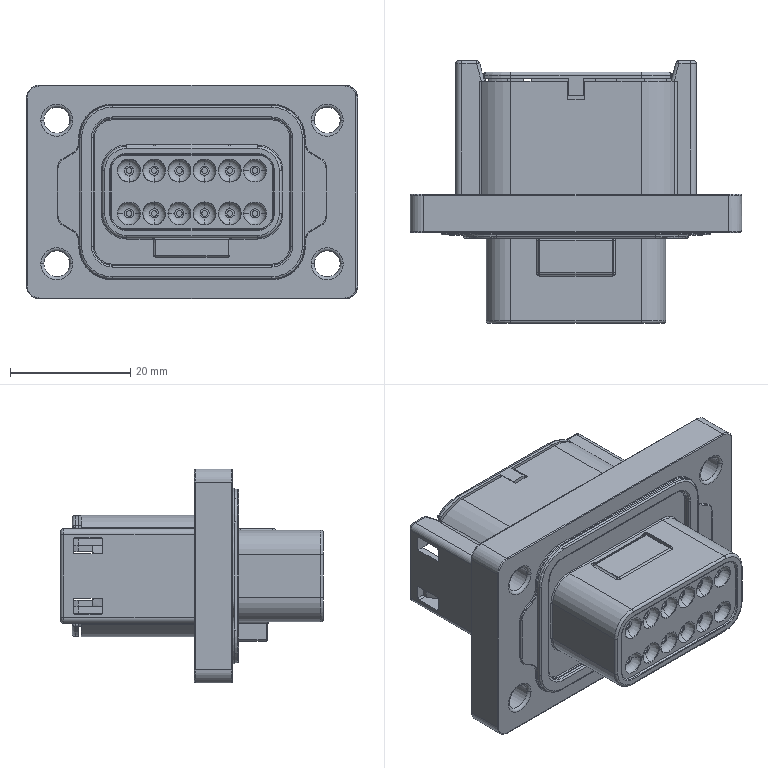Part | SolidWorks | features BaseBody 1 | 1 solid | 837 faces | box 55.12 x 43.688 x 35.56 mm | volume 26198 mm3 | plane 373 | cylinder 282 | torus 102 | cone 40 | sphere 28 | spline 12 | commonest cylinder face diameters 0.6 x66 0.94 x24 3.81 x24 0.3 x23 1 x22 9.56 x14